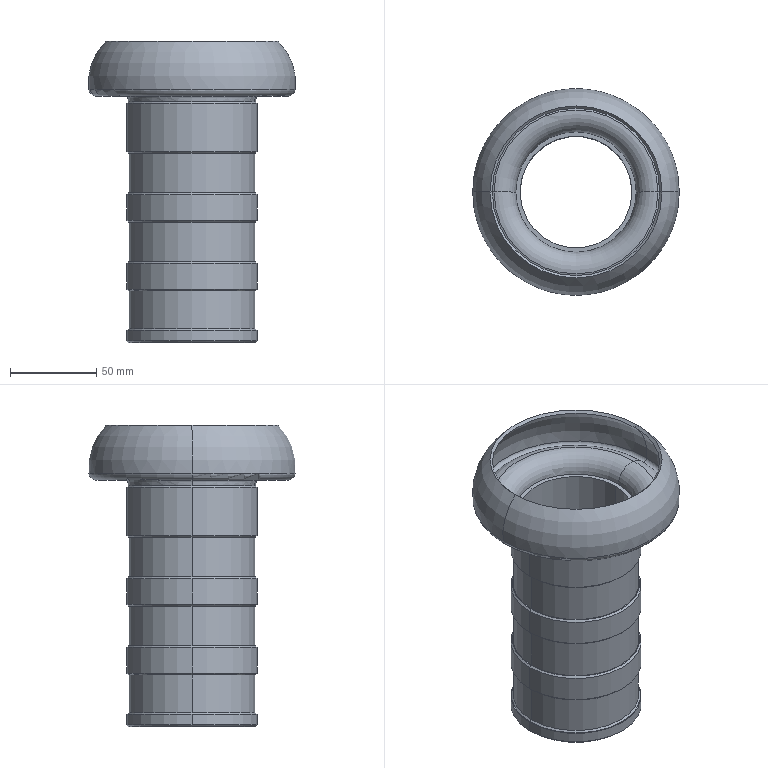Part | SolidWorks | features Chamfer 2, Extrusion 1, ICE 1, LPattern 1, Revolution 1 | 1 solid | 58 faces | box 120.458 x 120.458 x 175 mm | volume 185173 mm3 | cone 18 | torus 16 | cylinder 16 | plane 8 | commonest cylinder face diameters 76 x8 73 x6 65 x2
STEP:
#1=CARTESIAN_POINT('',(47.213,0.,148.274));
#2=VERTEX_POINT('',#1);
#3=CARTESIAN_POINT('',(-47.213,0.,148.274));
#4=VERTEX_POINT('',#3);
#5=CARTESIAN_POINT('',(0.,0.,148.274));
#6=DIRECTION('',(0.,0.,-1.));
#7=DIRECTION('',(-1.,0.,0.));
#8=AXIS2_PLACEMENT_3D('',#5,#6,#7);
#9=CIRCLE('',#8,47.213);
#10=EDGE_CURVE('',#2,#4,#9,.T.);
#11=ORIENTED_EDGE('',*,*,#10,.F.);
#12=CARTESIAN_POINT('',(54.205,0.,143.544));
#13=VERTEX_POINT('',#12);
#14=CARTESIAN_POINT('',(44.886,0.,137.301));
#15=DIRECTION('',(0.,1.,0.));
#16=DIRECTION('',(-1.,0.,0.));
#17=AXIS2_PLACEMENT_3D('',#14,#15,#16);
#18=CIRCLE('',#17,11.217);
#19=EDGE_CURVE('',#2,#13,#18,.T.);
#20=ORIENTED_EDGE('',*,*,#19,.T.);
#21=CARTESIAN_POINT('',(-54.205,0.,143.544));
#22=VERTEX_POINT('',#21);
#23=CARTESIAN_POINT('',(0.,0.,143.544));
#24=DIRECTION('',(0.,0.,-1.));
#25=DIRECTION('',(-1.,0.,0.));
#26=AXIS2_PLACEMENT_3D('',#23,#24,#25);
#27=CIRCLE('',#26,54.205);
#28=EDGE_CURVE('',#13,#22,#27,.T.);
#29=ORIENTED_EDGE('',*,*,#28,.T.);
#30=CARTESIAN_POINT('',(-44.886,0.,137.301));
#31=DIRECTION('',(0.,-1.,0.));
#32=DIRECTION('',(0.,0.,-1.));
#33=AXIS2_PLACEMENT_3D('',#30,#31,#32);
#34=CIRCLE('',#33,11.217);
#35=EDGE_CURVE('',#4,#22,#34,.T.);
#36=ORIENTED_EDGE('',*,*,#35,.F.);
#37=EDGE_LOOP('',(#11,#20,#29,#36));
#38=FACE_OUTER_BOUND('',#37,.T.);
#39=CARTESIAN_POINT('',(0.,0.,137.301));
#40=DIRECTION('',(0.,0.,-1.));
#41=DIRECTION('',(-1.,0.,0.));
#42=AXIS2_PLACEMENT_3D('',#39,#40,#41);
#43=TOROIDAL_SURFACE('',#42,44.886,11.217);
#44=ADVANCED_FACE('',(#38),#43,.F.);
#45=CARTESIAN_POINT('',(-60.,0.,147.099));
#46=VERTEX_POINT('',#45);
#47=CARTESIAN_POINT('',(60.,0.,147.099));
#48=VERTEX_POINT('',#47);
#49=CARTESIAN_POINT('',(0.,0.,147.099));
#50=DIRECTION('',(0.,0.,-1.));
#51=DIRECTION('',(-1.,0.,0.));
#52=AXIS2_PLACEMENT_3D('',#49,#50,#51);
#53=CIRCLE('',#52,60.);
#54=EDGE_CURVE('',#46,#48,#53,.T.);
#55=ORIENTED_EDGE('',*,*,#54,.T.);
#56=CARTESIAN_POINT('',(55.701,0.,147.606));
#57=DIRECTION('',(0.,1.,0.));
#58=DIRECTION('',(-1.,0.,0.));
#59=AXIS2_PLACEMENT_3D('',#56,#57,#58);
#60=CIRCLE('',#59,4.329);
#61=EDGE_CURVE('',#48,#13,#60,.T.);
#62=ORIENTED_EDGE('',*,*,#61,.T.);
#63=CARTESIAN_POINT('',(0.,0.,143.544));
#64=DIRECTION('',(0.,0.,-1.));
#65=DIRECTION('',(-1.,0.,0.));
#66=AXIS2_PLACEMENT_3D('',#63,#64,#65);
#67=CIRCLE('',#66,54.205);
#68=EDGE_CURVE('',#22,#13,#67,.T.);
#69=ORIENTED_EDGE('',*,*,#68,.F.);
#70=CARTESIAN_POINT('',(-55.701,0.,147.606));
#71=DIRECTION('',(0.,-1.,0.));
#72=DIRECTION('',(0.,0.,-1.));
#73=AXIS2_PLACEMENT_3D('',#70,#71,#72);
#74=CIRCLE('',#73,4.329);
#75=EDGE_CURVE('',#46,#22,#74,.T.);
#76=ORIENTED_EDGE('',*,*,#75,.F.);
#77=EDGE_LOOP('',(#55,#62,#69,#76));
#78=FACE_OUTER_BOUND('',#77,.T.);
#79=CARTESIAN_POINT('',(0.,0.,147.606));
#80=DIRECTION('',(0.,0.,-1.));
#81=DIRECTION('',(-1.,0.,0.));
#82=AXIS2_PLACEMENT_3D('',#79,#80,#81);
#83=TOROIDAL_SURFACE('',#82,55.701,4.329);
#84=ADVANCED_FACE('',(#78),#83,.T.);
#85=CARTESIAN_POINT('',(-50.,0.,175.));
#86=VERTEX_POINT('',#85);
#87=CARTESIAN_POINT('',(50.,0.,175.));
#88=VERTEX_POINT('',#87);
#89=CARTESIAN_POINT('',(0.,0.,175.));
#90=DIRECTION('',(0.,0.,-1.));
#91=DIRECTION('',(-1.,0.,0.));
#92=AXIS2_PLACEMENT_3D('',#89,#90,#91);
#93=CIRCLE('',#92,50.);
#94=EDGE_CURVE('',#86,#88,#93,.T.);
#95=ORIENTED_EDGE('',*,*,#94,.T.);
#96=CARTESIAN_POINT('',(26.951,0.,150.997));
#97=DIRECTION('',(0.,1.,0.));
#98=DIRECTION('',(-1.,0.,0.));
#99=AXIS2_PLACEMENT_3D('',#96,#97,#98);
#100=CIRCLE('',#99,33.278);
#101=EDGE_CURVE('',#88,#48,#100,.T.);
#102=ORIENTED_EDGE('',*,*,#101,.T.);
#103=ORIENTED_EDGE('',*,*,#54,.F.);
#104=CARTESIAN_POINT('',(-26.951,0.,150.997));
#105=DIRECTION('',(0.,-1.,0.));
#106=DIRECTION('',(0.,0.,-1.));
#107=AXIS2_PLACEMENT_3D('',#104,#105,#106);
#108=CIRCLE('',#107,33.278);
#109=EDGE_CURVE('',#86,#46,#108,.T.);
#110=ORIENTED_EDGE('',*,*,#109,.F.);
#111=EDGE_LOOP('',(#95,#102,#103,#110));
#112=FACE_OUTER_BOUND('',#111,.T.);
#113=CARTESIAN_POINT('',(0.,0.,150.997));
#114=DIRECTION('',(0.,0.,-1.));
#115=DIRECTION('',(-1.,0.,0.));
#116=AXIS2_PLACEMENT_3D('',#113,#114,#115);
#117=TOROIDAL_SURFACE('',#116,26.951,33.278);
#118=ADVANCED_FACE('',(#112),#117,.T.);
#119=CARTESIAN_POINT('',(48.615,0.,173.557));
#120=VERTEX_POINT('',#119);
#121=CARTESIAN_POINT('',(-48.615,0.,173.557));
#122=VERTEX_POINT('',#121);
#123=CARTESIAN_POINT('',(0.,0.,173.557));
#124=DIRECTION('',(0.,0.,-1.));
#125=DIRECTION('',(-1.,0.,0.));
#126=AXIS2_PLACEMENT_3D('',#123,#124,#125);
#127=CIRCLE('',#126,48.615);
#128=EDGE_CURVE('',#120,#122,#127,.T.);
#129=ORIENTED_EDGE('',*,*,#128,.T.);
#130=CARTESIAN_POINT('',(-48.615,0.,173.557));
#131=DIRECTION('',(-0.6926,0.,0.7213));
#132=VECTOR('',#131,1000.);
#133=LINE('',#130,#132);
#134=EDGE_CURVE('',#122,#86,#133,.T.);
#135=ORIENTED_EDGE('',*,*,#134,.T.);
#136=CARTESIAN_POINT('',(0.,0.,175.));
#137=DIRECTION('',(0.,0.,-1.));
#138=DIRECTION('',(-1.,0.,0.));
#139=AXIS2_PLACEMENT_3D('',#136,#137,#138);
#140=CIRCLE('',#139,50.);
#141=EDGE_CURVE('',#88,#86,#140,.T.);
#142=ORIENTED_EDGE('',*,*,#141,.F.);
#143=CARTESIAN_POINT('',(48.615,0.,173.557));
#144=DIRECTION('',(0.6926,0.,0.7213));
#145=VECTOR('',#144,1000.);
#146=LINE('',#143,#145);
#147=EDGE_CURVE('',#120,#88,#146,.T.);
#148=ORIENTED_EDGE('',*,*,#147,.F.);
#149=EDGE_LOOP('',(#129,#135,#142,#148));
#150=FACE_OUTER_BOUND('',#149,.T.);
#151=CARTESIAN_POINT('',(0.,0.,173.557));
#152=DIRECTION('',(0.,0.,1.));
#153=DIRECTION('',(1.,0.,0.));
#154=AXIS2_PLACEMENT_3D('',#151,#152,#153);
#155=CONICAL_SURFACE('',#154,48.615,0.7651);
#156=ADVANCED_FACE('',(#150),#155,.F.);
#157=ORIENTED_EDGE('',*,*,#128,.F.);
#158=CARTESIAN_POINT('',(58.014,0.,147.333));
#159=VERTEX_POINT('',#158);
#160=CARTESIAN_POINT('',(26.951,0.,150.997));
#161=DIRECTION('',(0.,1.,0.));
#162=DIRECTION('',(-1.,0.,0.));
#163=AXIS2_PLACEMENT_3D('',#160,#161,#162);
#164=CIRCLE('',#163,31.278);
#165=EDGE_CURVE('',#120,#159,#164,.T.);
#166=ORIENTED_EDGE('',*,*,#165,.T.);
#167=CARTESIAN_POINT('',(-58.014,0.,147.333));
#168=VERTEX_POINT('',#167);
#169=CARTESIAN_POINT('',(0.,0.,147.333));
#170=DIRECTION('',(0.,0.,-1.));
#171=DIRECTION('',(-1.,0.,0.));
#172=AXIS2_PLACEMENT_3D('',#169,#170,#171);
#173=CIRCLE('',#172,58.014);
#174=EDGE_CURVE('',#159,#168,#173,.T.);
#175=ORIENTED_EDGE('',*,*,#174,.T.);
#176=CARTESIAN_POINT('',(-26.951,0.,150.997));
#177=DIRECTION('',(0.,-1.,0.));
#178=DIRECTION('',(0.,0.,-1.));
#179=AXIS2_PLACEMENT_3D('',#176,#177,#178);
#180=CIRCLE('',#179,31.278);
#181=EDGE_CURVE('',#122,#168,#180,.T.);
#182=ORIENTED_EDGE('',*,*,#181,.F.);
#183=EDGE_LOOP('',(#157,#166,#175,#182));
#184=FACE_OUTER_BOUND('',#183,.T.);
#185=CARTESIAN_POINT('',(0.,0.,150.997));
#186=DIRECTION('',(0.,0.,-1.));
#187=DIRECTION('',(-1.,0.,0.));
#188=AXIS2_PLACEMENT_3D('',#185,#186,#187);
#189=TOROIDAL_SURFACE('',#188,26.951,31.278);
#190=ADVANCED_FACE('',(#184),#189,.F.);
#191=ORIENTED_EDGE('',*,*,#174,.F.);
#192=CARTESIAN_POINT('',(55.411,0.,145.295));
#193=VERTEX_POINT('',#192);
#194=CARTESIAN_POINT('',(55.701,0.,147.606));
#195=DIRECTION('',(0.,1.,0.));
#196=DIRECTION('',(-1.,0.,0.));
#197=AXIS2_PLACEMENT_3D('',#194,#195,#196);
#198=CIRCLE('',#197,2.329);
#199=EDGE_CURVE('',#159,#193,#198,.T.);
#200=ORIENTED_EDGE('',*,*,#199,.T.);
#201=CARTESIAN_POINT('',(-55.411,0.,145.295));
#202=VERTEX_POINT('',#201);
#203=CARTESIAN_POINT('',(0.,0.,145.295));
#204=DIRECTION('',(0.,0.,-1.));
#205=DIRECTION('',(-1.,0.,0.));
#206=AXIS2_PLACEMENT_3D('',#203,#204,#205);
#207=CIRCLE('',#206,55.411);
#208=EDGE_CURVE('',#193,#202,#207,.T.);
#209=ORIENTED_EDGE('',*,*,#208,.T.);
#210=CARTESIAN_POINT('',(-55.701,0.,147.606));
#211=DIRECTION('',(0.,-1.,0.));
#212=DIRECTION('',(0.,0.,-1.));
#213=AXIS2_PLACEMENT_3D('',#210,#211,#212);
#214=CIRCLE('',#213,2.329);
#215=EDGE_CURVE('',#168,#202,#214,.T.);
#216=ORIENTED_EDGE('',*,*,#215,.F.);
#217=EDGE_LOOP('',(#191,#200,#209,#216));
#218=FACE_OUTER_BOUND('',#217,.T.);
#219=CARTESIAN_POINT('',(0.,0.,147.606));
#220=DIRECTION('',(0.,0.,-1.));
#221=DIRECTION('',(-1.,0.,0.));
#222=AXIS2_PLACEMENT_3D('',#219,#220,#221);
#223=TOROIDAL_SURFACE('',#222,55.701,2.329);
#224=ADVANCED_FACE('',(#218),#223,.F.);
#225=CARTESIAN_POINT('',(-47.628,0.,150.231));
#226=VERTEX_POINT('',#225);
#227=CARTESIAN_POINT('',(47.628,0.,150.231));
#228=VERTEX_POINT('',#227);
#229=CARTESIAN_POINT('',(0.,0.,150.231));
#230=DIRECTION('',(0.,0.,-1.));
#231=DIRECTION('',(-1.,0.,0.));
#232=AXIS2_PLACEMENT_3D('',#229,#230,#231);
#233=CIRCLE('',#232,47.628);
#234=EDGE_CURVE('',#226,#228,#233,.T.);
#235=ORIENTED_EDGE('',*,*,#234,.T.);
#236=CARTESIAN_POINT('',(44.886,0.,137.301));
#237=DIRECTION('',(0.,1.,0.));
#238=DIRECTION('',(-1.,0.,0.));
#239=AXIS2_PLACEMENT_3D('',#236,#237,#238);
#240=CIRCLE('',#239,13.217);
#241=EDGE_CURVE('',#228,#193,#240,.T.);
#242=ORIENTED_EDGE('',*,*,#241,.T.);
#243=CARTESIAN_POINT('',(0.,0.,145.295));
#244=DIRECTION('',(0.,0.,-1.));
#245=DIRECTION('',(-1.,0.,0.));
#246=AXIS2_PLACEMENT_3D('',#243,#244,#245);
#247=CIRCLE('',#246,55.411);
#248=EDGE_CURVE('',#202,#193,#247,.T.);
#249=ORIENTED_EDGE('',*,*,#248,.F.);
#250=CARTESIAN_POINT('',(-44.886,0.,137.301));
#251=DIRECTION('',(0.,-1.,0.));
#252=DIRECTION('',(0.,0.,-1.));
#253=AXIS2_PLACEMENT_3D('',#250,#251,#252);
#254=CIRCLE('',#253,13.217);
#255=EDGE_CURVE('',#226,#202,#254,.T.);
#256=ORIENTED_EDGE('',*,*,#255,.F.);
#257=EDGE_LOOP('',(#235,#242,#249,#256));
#258=FACE_OUTER_BOUND('',#257,.T.);
#259=CARTESIAN_POINT('',(0.,0.,137.301));
#260=DIRECTION('',(0.,0.,-1.));
#261=DIRECTION('',(-1.,0.,0.));
#262=AXIS2_PLACEMENT_3D('',#259,#260,#261);
#263=TOROIDAL_SURFACE('',#262,44.886,13.217);
#264=ADVANCED_FACE('',(#258),#263,.T.);
#265=CARTESIAN_POINT('',(-35.,0.,140.));
#266=VERTEX_POINT('',#265);
#267=CARTESIAN_POINT('',(35.,0.,140.));
#268=VERTEX_POINT('',#267);
#269=CARTESIAN_POINT('',(0.,0.,140.));
#270=DIRECTION('',(0.,0.,-1.));
#271=DIRECTION('',(-1.,0.,0.));
#272=AXIS2_PLACEMENT_3D('',#269,#270,#271);
#273=CIRCLE('',#272,35.);
#274=EDGE_CURVE('',#266,#268,#273,.T.);
#275=ORIENTED_EDGE('',*,*,#274,.T.);
#276=CARTESIAN_POINT('',(45.458,0.,140.));
#277=DIRECTION('',(0.,1.,0.));
#278=DIRECTION('',(-1.,0.,0.));
#279=AXIS2_PLACEMENT_3D('',#276,#277,#278);
#280=CIRCLE('',#279,10.458);
#281=EDGE_CURVE('',#268,#228,#280,.T.);
#282=ORIENTED_EDGE('',*,*,#281,.T.);
#283=ORIENTED_EDGE('',*,*,#234,.F.);
#284=CARTESIAN_POINT('',(-45.458,0.,140.));
#285=DIRECTION('',(0.,-1.,0.));
#286=DIRECTION('',(0.,0.,-1.));
#287=AXIS2_PLACEMENT_3D('',#284,#285,#286);
#288=CIRCLE('',#287,10.458);
#289=EDGE_CURVE('',#266,#226,#288,.T.);
#290=ORIENTED_EDGE('',*,*,#289,.F.);
#291=EDGE_LOOP('',(#275,#282,#283,#290));
#292=FACE_OUTER_BOUND('',#291,.T.);
#293=CARTESIAN_POINT('',(0.,0.,140.));
#294=DIRECTION('',(0.,0.,-1.));
#295=DIRECTION('',(-1.,0.,0.));
#296=AXIS2_PLACEMENT_3D('',#293,#294,#295);
#297=TOROIDAL_SURFACE('',#296,45.458,10.458);
#298=ADVANCED_FACE('',(#292),#297,.T.);
#299=CARTESIAN_POINT('',(-37.,0.,140.));
#300=VERTEX_POINT('',#299);
#301=CARTESIAN_POINT('',(37.,0.,140.));
#302=VERTEX_POINT('',#301);
#303=CARTESIAN_POINT('',(0.,0.,140.));
#304=DIRECTION('',(0.,0.,1.));
#305=DIRECTION('',(1.,0.,0.));
#306=AXIS2_PLACEMENT_3D('',#303,#304,#305);
#307=CIRCLE('',#306,37.);
#308=EDGE_CURVE('',#300,#302,#307,.T.);
#309=ORIENTED_EDGE('',*,*,#308,.T.);
#310=CARTESIAN_POINT('',(45.458,0.,140.));
#311=DIRECTION('',(0.,1.,0.));
#312=DIRECTION('',(-1.,0.,0.));
#313=AXIS2_PLACEMENT_3D('',#310,#311,#312);
#314=CIRCLE('',#313,8.458);
#315=EDGE_CURVE('',#302,#2,#314,.T.);
#316=ORIENTED_EDGE('',*,*,#315,.T.);
#317=ORIENTED_EDGE('',*,*,#10,.T.);
#318=CARTESIAN_POINT('',(-45.458,0.,140.));
#319=DIRECTION('',(0.,-1.,0.));
#320=DIRECTION('',(0.,0.,-1.));
#321=AXIS2_PLACEMENT_3D('',#318,#319,#320);
#322=CIRCLE('',#321,8.458);
#323=EDGE_CURVE('',#300,#4,#322,.T.);
#324=ORIENTED_EDGE('',*,*,#323,.F.);
#325=EDGE_LOOP('',(#309,#316,#317,#324));
#326=FACE_OUTER_BOUND('',#325,.T.);
#327=CARTESIAN_POINT('',(0.,0.,140.));
#328=DIRECTION('',(0.,0.,-1.));
#329=DIRECTION('',(-1.,0.,0.));
#330=AXIS2_PLACEMENT_3D('',#327,#328,#329);
#331=TOROIDAL_SURFACE('',#330,45.458,8.458);
#332=ADVANCED_FACE('',(#326),#331,.F.);
#333=CARTESIAN_POINT('',(-37.,0.,110.));
#334=VERTEX_POINT('',#333);
#335=CARTESIAN_POINT('',(37.,0.,110.));
#336=VERTEX_POINT('',#335);
#337=CARTESIAN_POINT('',(0.,0.,110.));
#338=DIRECTION('',(0.,0.,-1.));
#339=DIRECTION('',(1.,0.,0.));
#340=AXIS2_PLACEMENT_3D('',#337,#338,#339);
#341=CIRCLE('',#340,37.);
#342=EDGE_CURVE('',#334,#336,#341,.T.);
#343=ORIENTED_EDGE('',*,*,#342,.F.);
#344=CARTESIAN_POINT('',(-38.,0.,111.));
#345=VERTEX_POINT('',#344);
#346=CARTESIAN_POINT('',(-38.,0.,111.));
#347=DIRECTION('',(-0.7071,0.,0.7071));
#348=VECTOR('',#347,1000.);
#349=LINE('',#346,#348);
#350=EDGE_CURVE('',#334,#345,#349,.T.);
#351=ORIENTED_EDGE('',*,*,#350,.T.);
#352=CARTESIAN_POINT('',(38.,0.,111.));
#353=VERTEX_POINT('',#352);
#354=CARTESIAN_POINT('',(0.,0.,111.));
#355=DIRECTION('',(0.,0.,1.));
#356=DIRECTION('',(1.,0.,0.));
#357=AXIS2_PLACEMENT_3D('',#354,#355,#356);
#358=CIRCLE('',#357,38.);
#359=EDGE_CURVE('',#353,#345,#358,.T.);
#360=ORIENTED_EDGE('',*,*,#359,.F.);
#361=CARTESIAN_POINT('',(38.,0.,111.));
#362=DIRECTION('',(0.7071,0.,0.7071));
#363=VECTOR('',#362,1000.);
#364=LINE('',#361,#363);
#365=EDGE_CURVE('',#336,#353,#364,.T.);
#366=ORIENTED_EDGE('',*,*,#365,.F.);
#367=EDGE_LOOP('',(#343,#351,#360,#366));
#368=FACE_OUTER_BOUND('',#367,.T.);
#369=CARTESIAN_POINT('',(0.,0.,111.));
#370=DIRECTION('',(0.,0.,1.));
#371=DIRECTION('',(1.,0.,0.));
#372=AXIS2_PLACEMENT_3D('',#369,#370,#371);
#373=CONICAL_SURFACE('',#372,38.,0.7854);
#374=ADVANCED_FACE('',(#368),#373,.T.);
#375=CARTESIAN_POINT('',(37.,0.,87.));
#376=VERTEX_POINT('',#375);
#377=CARTESIAN_POINT('',(-37.,0.,87.));
#378=VERTEX_POINT('',#377);
#379=CARTESIAN_POINT('',(0.,0.,87.));
#380=DIRECTION('',(0.,0.,1.));
#381=DIRECTION('',(1.,0.,0.));
#382=AXIS2_PLACEMENT_3D('',#379,#380,#381);
#383=CIRCLE('',#382,37.);
#384=EDGE_CURVE('',#376,#378,#383,.T.);
#385=ORIENTED_EDGE('',*,*,#384,.F.);
#386=CARTESIAN_POINT('',(38.,0.,86.));
#387=VERTEX_POINT('',#386);
#388=CARTESIAN_POINT('',(37.,0.,87.));
#389=DIRECTION('',(0.7071,0.,-0.7071));
#390=VECTOR('',#389,1000.);
#391=LINE('',#388,#390);
#392=EDGE_CURVE('',#376,#387,#391,.T.);
#393=ORIENTED_EDGE('',*,*,#392,.T.);
#394=CARTESIAN_POINT('',(-38.,0.,86.));
#395=VERTEX_POINT('',#394);
#396=CARTESIAN_POINT('',(0.,0.,86.));
#397=DIRECTION('',(0.,0.,-1.));
#398=DIRECTION('',(1.,0.,0.));
#399=AXIS2_PLACEMENT_3D('',#396,#397,#398);
#400=CIRCLE('',#399,38.);
#401=EDGE_CURVE('',#395,#387,#400,.T.);
#402=ORIENTED_EDGE('',*,*,#401,.F.);
#403=CARTESIAN_POINT('',(-37.,0.,87.));
#404=DIRECTION('',(-0.7071,0.,-0.7071));
#405=VECTOR('',#404,1000.);
#406=LINE('',#403,#405);
#407=EDGE_CURVE('',#378,#395,#406,.T.);
#408=ORIENTED_EDGE('',*,*,#407,.F.);
#409=EDGE_LOOP('',(#385,#393,#402,#408));
#410=FACE_OUTER_BOUND('',#409,.T.);
#411=CARTESIAN_POINT('',(0.,0.,87.));
#412=DIRECTION('',(0.,0.,-1.));
#413=DIRECTION('',(-1.,0.,0.));
#414=AXIS2_PLACEMENT_3D('',#411,#412,#413);
#415=CONICAL_SURFACE('',#414,37.,0.7854);
#416=ADVANCED_FACE('',(#410),#415,.T.);
#417=CARTESIAN_POINT('',(-37.,0.,70.));
#418=VERTEX_POINT('',#417);
#419=CARTESIAN_POINT('',(37.,0.,70.));
#420=VERTEX_POINT('',#419);
#421=CARTESIAN_POINT('',(0.,0.,70.));
#422=DIRECTION('',(0.,0.,-1.));
#423=DIRECTION('',(1.,0.,0.));
#424=AXIS2_PLACEMENT_3D('',#421,#422,#423);
#425=CIRCLE('',#424,37.);
#426=EDGE_CURVE('',#418,#420,#425,.T.);
#427=ORIENTED_EDGE('',*,*,#426,.F.);
#428=CARTESIAN_POINT('',(-38.,0.,71.));
#429=VERTEX_POINT('',#428);
#430=CARTESIAN_POINT('',(-38.,0.,71.));
#431=DIRECTION('',(-0.7071,0.,0.7071));
#432=VECTOR('',#431,1000.);
#433=LINE('',#430,#432);
#434=EDGE_CURVE('',#418,#429,#433,.T.);
#435=ORIENTED_EDGE('',*,*,#434,.T.);
#436=CARTESIAN_POINT('',(38.,0.,71.));
#437=VERTEX_POINT('',#436);
#438=CARTESIAN_POINT('',(0.,0.,71.));
#439=DIRECTION('',(0.,0.,1.));
#440=DIRECTION('',(1.,0.,0.));
#441=AXIS2_PLACEMENT_3D('',#438,#439,#440);
#442=CIRCLE('',#441,38.);
#443=EDGE_CURVE('',#437,#429,#442,.T.);
#444=ORIENTED_EDGE('',*,*,#443,.F.);
#445=CARTESIAN_POINT('',(38.,0.,71.));
#446=DIRECTION('',(0.7071,0.,0.7071));
#447=VECTOR('',#446,1000.);
#448=LINE('',#445,#447);
#449=EDGE_CURVE('',#420,#437,#448,.T.);
#450=ORIENTED_EDGE('',*,*,#449,.F.);
#451=EDGE_LOOP('',(#427,#435,#444,#450));
#452=FACE_OUTER_BOUND('',#451,.T.);
#453=CARTESIAN_POINT('',(0.,0.,71.));
#454=DIRECTION('',(0.,0.,1.));
#455=DIRECTION('',(1.,0.,0.));
#456=AXIS2_PLACEMENT_3D('',#453,#454,#455);
#457=CONICAL_SURFACE('',#456,38.,0.7854);
#458=ADVANCED_FACE('',(#452),#457,.T.);
#459=CARTESIAN_POINT('',(37.,0.,47.));
#460=VERTEX_POINT('',#459);
#461=CARTESIAN_POINT('',(-37.,0.,47.));
#462=VERTEX_POINT('',#461);
#463=CARTESIAN_POINT('',(0.,0.,47.));
#464=DIRECTION('',(0.,0.,1.));
#465=DIRECTION('',(1.,0.,0.));
#466=AXIS2_PLACEMENT_3D('',#463,#464,#465);
#467=CIRCLE('',#466,37.);
#468=EDGE_CURVE('',#460,#462,#467,.T.);
#469=ORIENTED_EDGE('',*,*,#468,.F.);
#470=CARTESIAN_POINT('',(38.,0.,46.));
#471=VERTEX_POINT('',#470);
#472=CARTESIAN_POINT('',(37.,0.,47.));
#473=DIRECTION('',(0.7071,0.,-0.7071));
#474=VECTOR('',#473,1000.);
#475=LINE('',#472,#474);
#476=EDGE_CURVE('',#460,#471,#475,.T.);
#477=ORIENTED_EDGE('',*,*,#476,.T.);
#478=CARTESIAN_POINT('',(-38.,0.,46.));
#479=VERTEX_POINT('',#478);
#480=CARTESIAN_POINT('',(0.,0.,46.));
#481=DIRECTION('',(0.,0.,-1.));
#482=DIRECTION('',(1.,0.,0.));
#483=AXIS2_PLACEMENT_3D('',#480,#481,#482);
#484=CIRCLE('',#483,38.);
#485=EDGE_CURVE('',#479,#471,#484,.T.);
#486=ORIENTED_EDGE('',*,*,#485,.F.);
#487=CARTESIAN_POINT('',(-37.,0.,47.));
#488=DIRECTION('',(-0.7071,0.,-0.7071));
#489=VECTOR('',#488,1000.);
#490=LINE('',#487,#489);
#491=EDGE_CURVE('',#462,#479,#490,.T.);
#492=ORIENTED_EDGE('',*,*,#491,.F.);
#493=EDGE_LOOP('',(#469,#477,#486,#492));
#494=FACE_OUTER_BOUND('',#493,.T.);
#495=CARTESIAN_POINT('',(0.,0.,47.));
#496=DIRECTION('',(0.,0.,-1.));
#497=DIRECTION('',(-1.,0.,0.));
#498=AXIS2_PLACEMENT_3D('',#495,#496,#497);
#499=CONICAL_SURFACE('',#498,37.,0.7854);
#500=ADVANCED_FACE('',(#494),#499,.T.);
#501=CARTESIAN_POINT('',(-37.,0.,30.));
#502=VERTEX_POINT('',#501);
#503=CARTESIAN_POINT('',(37.,0.,30.));
#504=VERTEX_POINT('',#503);
#505=CARTESIAN_POINT('',(0.,0.,30.));
#506=DIRECTION('',(0.,0.,-1.));
#507=DIRECTION('',(1.,0.,0.));
#508=AXIS2_PLACEMENT_3D('',#505,#506,#507);
#509=CIRCLE('',#508,37.);
#510=EDGE_CURVE('',#502,#504,#509,.T.);
#511=ORIENTED_EDGE('',*,*,#510,.F.);
#512=CARTESIAN_POINT('',(-38.,0.,31.));
#513=VERTEX_POINT('',#512);
#514=CARTESIAN_POINT('',(-38.,0.,31.));
#515=DIRECTION('',(-0.7071,0.,0.7071));
#516=VECTOR('',#515,1000.);
#517=LINE('',#514,#516);
#518=EDGE_CURVE('',#502,#513,#517,.T.);
#519=ORIENTED_EDGE('',*,*,#518,.T.);
#520=CARTESIAN_POINT('',(38.,0.,31.));
#521=VERTEX_POINT('',#520);
#522=CARTESIAN_POINT('',(0.,0.,31.));
#523=DIRECTION('',(0.,0.,1.));
#524=DIRECTION('',(1.,0.,0.));
#525=AXIS2_PLACEMENT_3D('',#522,#523,#524);
#526=CIRCLE('',#525,38.);
#527=EDGE_CURVE('',#521,#513,#526,.T.);
#528=ORIENTED_EDGE('',*,*,#527,.F.);
#529=CARTESIAN_POINT('',(38.,0.,31.));
#530=DIRECTION('',(0.7071,0.,0.7071));
#531=VECTOR('',#530,1000.);
#532=LINE('',#529,#531);
#533=EDGE_CURVE('',#504,#521,#532,.T.);
#534=ORIENTED_EDGE('',*,*,#533,.F.);
#535=EDGE_LOOP('',(#511,#519,#528,#534));
#536=FACE_OUTER_BOUND('',#535,.T.);
#537=CARTESIAN_POINT('',(0.,0.,31.));
#538=DIRECTION('',(0.,0.,1.));
#539=DIRECTION('',(1.,0.,0.));
#540=AXIS2_PLACEMENT_3D('',#537,#538,#539);
#541=CONICAL_SURFACE('',#540,38.,0.7854);
#542=ADVANCED_FACE('',(#536),#541,.T.);
#543=CARTESIAN_POINT('',(36.5,0.,8.));
#544=VERTEX_POINT('',#543);
#545=CARTESIAN_POINT('',(-36.5,0.,8.));
#546=VERTEX_POINT('',#545);
#547=CARTESIAN_POINT('',(0.,0.,8.));
#548=DIRECTION('',(0.,0.,1.));
#549=DIRECTION('',(1.,0.,0.));
#550=AXIS2_PLACEMENT_3D('',#547,#548,#549);
#551=CIRCLE('',#550,36.5);
#552=EDGE_CURVE('',#544,#546,#551,.T.);
#553=ORIENTED_EDGE('',*,*,#552,.F.);
#554=CARTESIAN_POINT('',(37.5,0.,7.));
#555=VERTEX_POINT('',#554);
#556=CARTESIAN_POINT('',(36.5,0.,8.));
#557=DIRECTION('',(0.7071,0.,-0.7071));
#558=VECTOR('',#557,1000.);
#559=LINE('',#556,#558);
#560=EDGE_CURVE('',#544,#555,#559,.T.);
#561=ORIENTED_EDGE('',*,*,#560,.T.);
#562=CARTESIAN_POINT('',(-37.5,0.,7.));
#563=VERTEX_POINT('',#562);
#564=CARTESIAN_POINT('',(0.,0.,7.));
#565=DIRECTION('',(0.,0.,-1.));
#566=DIRECTION('',(1.,0.,0.));
#567=AXIS2_PLACEMENT_3D('',#564,#565,#566);
#568=CIRCLE('',#567,37.5);
#569=EDGE_CURVE('',#563,#555,#568,.T.);
#570=ORIENTED_EDGE('',*,*,#569,.F.);
#571=CARTESIAN_POINT('',(-36.5,0.,8.));
#572=DIRECTION('',(-0.7071,0.,-0.7071));
#573=VECTOR('',#572,1000.);
#574=LINE('',#571,#573);
#575=EDGE_CURVE('',#546,#563,#574,.T.);
#576=ORIENTED_EDGE('',*,*,#575,.F.);
#577=EDGE_LOOP('',(#553,#561,#570,#576));
#578=FACE_OUTER_BOUND('',#577,.T.);
#579=CARTESIAN_POINT('',(0.,0.,8.));
#580=DIRECTION('',(0.,0.,-1.));
#581=DIRECTION('',(-1.,0.,0.));
#582=AXIS2_PLACEMENT_3D('',#579,#580,#581);
#583=CONICAL_SURFACE('',#582,36.5,0.7854);
#584=ADVANCED_FACE('',(#578),#583,.T.);
#585=CARTESIAN_POINT('',(-37.,0.,0.));
#586=VERTEX_POINT('',#585);
#587=CARTESIAN_POINT('',(37.,0.,0.));
#588=VERTEX_POINT('',#587);
#589=CARTESIAN_POINT('',(0.,0.,0.));
#590=DIRECTION('',(0.,0.,-1.));
#591=DIRECTION('',(1.,0.,0.));
#592=AXIS2_PLACEMENT_3D('',#589,#590,#591);
#593=CIRCLE('',#592,37.);
#594=EDGE_CURVE('',#586,#588,#593,.T.);
#595=ORIENTED_EDGE('',*,*,#594,.F.);
#596=CARTESIAN_POINT('',(-38.,0.,1.));
#597=VERTEX_POINT('',#596);
#598=CARTESIAN_POINT('',(-38.,0.,1.));
#599=DIRECTION('',(-0.7071,0.,0.7071));
#600=VECTOR('',#599,1000.);
#601=LINE('',#598,#600);
#602=EDGE_CURVE('',#586,#597,#601,.T.);
#603=ORIENTED_EDGE('',*,*,#602,.T.);
#604=CARTESIAN_POINT('',(38.,0.,1.));
#605=VERTEX_POINT('',#604);
#606=CARTESIAN_POINT('',(0.,0.,1.));
#607=DIRECTION('',(0.,0.,1.));
#608=DIRECTION('',(1.,0.,0.));
#609=AXIS2_PLACEMENT_3D('',#606,#607,#608);
#610=CIRCLE('',#609,38.);
#611=EDGE_CURVE('',#605,#597,#610,.T.);
#612=ORIENTED_EDGE('',*,*,#611,.F.);
#613=CARTESIAN_POINT('',(38.,0.,1.));
#614=DIRECTION('',(0.7071,0.,0.7071));
#615=VECTOR('',#614,1000.);
#616=LINE('',#613,#615);
#617=EDGE_CURVE('',#588,#605,#616,.T.);
#618=ORIENTED_EDGE('',*,*,#617,.F.);
#619=EDGE_LOOP('',(#595,#603,#612,#618));
#620=FACE_OUTER_BOUND('',#619,.T.);
#621=CARTESIAN_POINT('',(0.,0.,1.));
#622=DIRECTION('',(0.,0.,1.));
#623=DIRECTION('',(1.,0.,0.));
#624=AXIS2_PLACEMENT_3D('',#621,#622,#623);
#625=CONICAL_SURFACE('',#624,38.,0.7854);
#626=ADVANCED_FACE('',(#620),#625,.T.);
#627=ORIENTED_EDGE('',*,*,#485,.T.);
#628=CARTESIAN_POINT('',(38.,0.,140.));
#629=DIRECTION('',(0.,0.,-1.));
#630=VECTOR('',#629,1000.);
#631=LINE('',#628,#630);
#632=EDGE_CURVE('',#471,#521,#631,.T.);
#633=ORIENTED_EDGE('',*,*,#632,.T.);
#634=ORIENTED_EDGE('',*,*,#527,.T.);
#635=CARTESIAN_POINT('',(-38.,0.,140.));
#636=DIRECTION('',(0.,0.,-1.));
#637=VECTOR('',#636,1000.);
#638=LINE('',#635,#637);
#639=EDGE_CURVE('',#479,#513,#638,.T.);
#640=ORIENTED_EDGE('',*,*,#639,.F.);
#641=EDGE_LOOP('',(#627,#633,#634,#640));
#642=FACE_OUTER_BOUND('',#641,.T.);
#643=CARTESIAN_POINT('',(0.,0.,140.));
#644=DIRECTION('',(0.,0.,-1.));
#645=DIRECTION('',(-1.,0.,0.));
#646=AXIS2_PLACEMENT_3D('',#643,#644,#645);
#647=CYLINDRICAL_SURFACE('',#646,38.);
#648=ADVANCED_FACE('',(#642),#647,.T.);
#649=CARTESIAN_POINT('',(36.5,0.,47.));
#650=VERTEX_POINT('',#649);
#651=CARTESIAN_POINT('',(-36.5,0.,47.));
#652=VERTEX_POINT('',#651);
#653=CARTESIAN_POINT('',(0.,0.,47.));
#654=DIRECTION('',(0.,0.,1.));
#655=DIRECTION('',(1.,0.,0.));
#656=AXIS2_PLACEMENT_3D('',#653,#654,#655);
#657=CIRCLE('',#656,36.5);
#658=EDGE_CURVE('',#650,#652,#657,.T.);
#659=ORIENTED_EDGE('',*,*,#658,.T.);
#660=CARTESIAN_POINT('',(-36.5,0.,70.));
#661=VERTEX_POINT('',#660);
#662=CARTESIAN_POINT('',(-36.5,0.,47.));
#663=DIRECTION('',(0.,0.,1.));
#664=VECTOR('',#663,1000.);
#665=LINE('',#662,#664);
#666=EDGE_CURVE('',#652,#661,#665,.T.);
#667=ORIENTED_EDGE('',*,*,#666,.T.);
#668=CARTESIAN_POINT('',(36.5,0.,70.));
#669=VERTEX_POINT('',#668);
#670=CARTESIAN_POINT('',(0.,0.,70.));
#671=DIRECTION('',(0.,0.,1.));
#672=DIRECTION('',(1.,0.,0.));
#673=AXIS2_PLACEMENT_3D('',#670,#671,#672);
#674=CIRCLE('',#673,36.5);
#675=EDGE_CURVE('',#669,#661,#674,.T.);
#676=ORIENTED_EDGE('',*,*,#675,.F.);
#677=CARTESIAN_POINT('',(36.5,0.,47.));
#678=DIRECTION('',(0.,0.,1.));
#679=VECTOR('',#678,1000.);
#680=LINE('',#677,#679);
#681=EDGE_CURVE('',#650,#669,#680,.T.);
#682=ORIENTED_EDGE('',*,*,#681,.F.);
#683=EDGE_LOOP('',(#659,#667,#676,#682));
#684=FACE_OUTER_BOUND('',#683,.T.);
#685=CARTESIAN_POINT('',(0.,0.,47.));
#686=DIRECTION('',(0.,0.,1.));
#687=DIRECTION('',(1.,0.,0.));
#688=AXIS2_PLACEMENT_3D('',#685,#686,#687);
#689=CYLINDRICAL_SURFACE('',#688,36.5);
#690=ADVANCED_FACE('',(#684),#689,.T.);
#691=ORIENTED_EDGE('',*,*,#552,.T.);
#692=CARTESIAN_POINT('',(-36.5,0.,30.));
#693=VERTEX_POINT('',#692);
#694=CARTESIAN_POINT('',(-36.5,0.,7.));
#695=DIRECTION('',(0.,0.,1.));
#696=VECTOR('',#695,1000.);
#697=LINE('',#694,#696);
#698=EDGE_CURVE('',#546,#693,#697,.T.);
#699=ORIENTED_EDGE('',*,*,#698,.T.);
#700=CARTESIAN_POINT('',(36.5,0.,30.));
#701=VERTEX_POINT('',#700);
#702=CARTESIAN_POINT('',(0.,0.,30.));
#703=DIRECTION('',(0.,0.,1.));
#704=DIRECTION('',(1.,0.,0.));
#705=AXIS2_PLACEMENT_3D('',#702,#703,#704);
#706=CIRCLE('',#705,36.5);
#707=EDGE_CURVE('',#701,#693,#706,.T.);
#708=ORIENTED_EDGE('',*,*,#707,.F.);
#709=CARTESIAN_POINT('',(36.5,0.,7.));
#710=DIRECTION('',(0.,0.,1.));
#711=VECTOR('',#710,1000.);
#712=LINE('',#709,#711);
#713=EDGE_CURVE('',#544,#701,#712,.T.);
#714=ORIENTED_EDGE('',*,*,#713,.F.);
#715=EDGE_LOOP('',(#691,#699,#708,#714));
#716=FACE_OUTER_BOUND('',#715,.T.);
#717=CARTESIAN_POINT('',(0.,0.,7.));
#718=DIRECTION('',(0.,0.,1.));
#719=DIRECTION('',(1.,0.,0.));
#720=AXIS2_PLACEMENT_3D('',#717,#718,#719);
#721=CYLINDRICAL_SURFACE('',#720,36.5);
#722=ADVANCED_FACE('',(#716),#721,.T.);
#723=CARTESIAN_POINT('',(36.5,0.,87.));
#724=VERTEX_POINT('',#723);
#725=CARTESIAN_POINT('',(-36.5,0.,87.));
#726=VERTEX_POINT('',#725);
#727=CARTESIAN_POINT('',(0.,0.,87.));
#728=DIRECTION('',(0.,0.,1.));
#729=DIRECTION('',(1.,0.,0.));
#730=AXIS2_PLACEMENT_3D('',#727,#728,#729);
#731=CIRCLE('',#730,36.5);
#732=EDGE_CURVE('',#724,#726,#731,.T.);
#733=ORIENTED_EDGE('',*,*,#732,.T.);
#734=CARTESIAN_POINT('',(-36.5,0.,110.));
#735=VERTEX_POINT('',#734);
#736=CARTESIAN_POINT('',(-36.5,0.,87.));
#737=DIRECTION('',(0.,0.,1.));
#738=VECTOR('',#737,1000.);
#739=LINE('',#736,#738);
#740=EDGE_CURVE('',#726,#735,#739,.T.);
#741=ORIENTED_EDGE('',*,*,#740,.T.);
#742=CARTESIAN_POINT('',(36.5,0.,110.));
#743=VERTEX_POINT('',#742);
#744=CARTESIAN_POINT('',(0.,0.,110.));
#745=DIRECTION('',(0.,0.,1.));
#746=DIRECTION('',(1.,0.,0.));
#747=AXIS2_PLACEMENT_3D('',#744,#745,#746);
#748=CIRCLE('',#747,36.5);
#749=EDGE_CURVE('',#743,#735,#748,.T.);
#750=ORIENTED_EDGE('',*,*,#749,.F.);
#751=CARTESIAN_POINT('',(36.5,0.,87.));
#752=DIRECTION('',(0.,0.,1.));
#753=VECTOR('',#752,1000.);
#754=LINE('',#751,#753);
#755=EDGE_CURVE('',#724,#743,#754,.T.);
#756=ORIENTED_EDGE('',*,*,#755,.F.);
#757=EDGE_LOOP('',(#733,#741,#750,#756));
#758=FACE_OUTER_BOUND('',#757,.T.);
#759=CARTESIAN_POINT('',(0.,0.,87.));
#760=DIRECTION('',(0.,0.,1.));
#761=DIRECTION('',(1.,0.,0.));
#762=AXIS2_PLACEMENT_3D('',#759,#760,#761);
#763=CYLINDRICAL_SURFACE('',#762,36.5);
#764=ADVANCED_FACE('',(#758),#763,.T.);
#765=CARTESIAN_POINT('',(0.,0.,140.));
#766=DIRECTION('',(0.,0.,1.));
#767=DIRECTION('',(1.,0.,0.));
#768=AXIS2_PLACEMENT_3D('',#765,#766,#767);
#769=CIRCLE('',#768,37.);
#770=EDGE_CURVE('',#302,#300,#769,.T.);
#771=ORIENTED_EDGE('',*,*,#770,.F.);
#772=CARTESIAN_POINT('',(38.,0.,139.));
#773=VERTEX_POINT('',#772);
#774=CARTESIAN_POINT('',(37.,0.,140.));
#775=DIRECTION('',(0.7071,0.,-0.7071));
#776=VECTOR('',#775,1000.);
#777=LINE('',#774,#776);
#778=EDGE_CURVE('',#302,#773,#777,.T.);
#779=ORIENTED_EDGE('',*,*,#778,.T.);
#780=CARTESIAN_POINT('',(-38.,0.,139.));
#781=VERTEX_POINT('',#780);
#782=CARTESIAN_POINT('',(0.,0.,139.));
#783=DIRECTION('',(0.,0.,-1.));
#784=DIRECTION('',(1.,0.,0.));
#785=AXIS2_PLACEMENT_3D('',#782,#783,#784);
#786=CIRCLE('',#785,38.);
#787=EDGE_CURVE('',#781,#773,#786,.T.);
#788=ORIENTED_EDGE('',*,*,#787,.F.);
#789=CARTESIAN_POINT('',(-37.,0.,140.));
#790=DIRECTION('',(-0.7071,0.,-0.7071));
#791=VECTOR('',#790,1000.);
#792=LINE('',#789,#791);
#793=EDGE_CURVE('',#300,#781,#792,.T.);
#794=ORIENTED_EDGE('',*,*,#793,.F.);
#795=EDGE_LOOP('',(#771,#779,#788,#794));
#796=FACE_OUTER_BOUND('',#795,.T.);
#797=CARTESIAN_POINT('',(0.,0.,140.));
#798=DIRECTION('',(0.,0.,-1.));
#799=DIRECTION('',(-1.,0.,0.));
#800=AXIS2_PLACEMENT_3D('',#797,#798,#799);
#801=CONICAL_SURFACE('',#800,37.,0.7854);
#802=ADVANCED_FACE('',(#796),#801,.T.);
#803=CARTESIAN_POINT('',(-32.5,0.,140.));
#804=VERTEX_POINT('',#803);
#805=CARTESIAN_POINT('',(32.5,0.,140.));
#806=VERTEX_POINT('',#805);
#807=CARTESIAN_POINT('',(0.,0.,140.));
#808=DIRECTION('',(0.,0.,1.));
#809=DIRECTION('',(1.,0.,0.));
#810=AXIS2_PLACEMENT_3D('',#807,#808,#809);
#811=CIRCLE('',#810,32.5);
#812=EDGE_CURVE('',#804,#806,#811,.T.);
#813=ORIENTED_EDGE('',*,*,#812,.T.);
#814=CARTESIAN_POINT('',(32.5,0.,0.));
#815=VERTEX_POINT('',#814);
#816=CARTESIAN_POINT('',(32.5,0.,140.));
#817=DIRECTION('',(0.,0.,-1.));
#818=VECTOR('',#817,1000.);
#819=LINE('',#816,#818);
#820=EDGE_CURVE('',#806,#815,#819,.T.);
#821=ORIENTED_EDGE('',*,*,#820,.T.);
#822=CARTESIAN_POINT('',(-32.5,0.,0.));
#823=VERTEX_POINT('',#822);
#824=CARTESIAN_POINT('',(0.,0.,0.));
#825=DIRECTION('',(0.,0.,1.));
#826=DIRECTION('',(1.,0.,0.));
#827=AXIS2_PLACEMENT_3D('',#824,#825,#826);
#828=CIRCLE('',#827,32.5);
#829=EDGE_CURVE('',#823,#815,#828,.T.);
#830=ORIENTED_EDGE('',*,*,#829,.F.);
#831=CARTESIAN_POINT('',(-32.5,0.,140.));
#832=DIRECTION('',(0.,0.,-1.));
#833=VECTOR('',#832,1000.);
#834=LINE('',#831,#833);
#835=EDGE_CURVE('',#804,#823,#834,.T.);
#836=ORIENTED_EDGE('',*,*,#835,.F.);
#837=EDGE_LOOP('',(#813,#821,#830,#836));
#838=FACE_OUTER_BOUND('',#837,.T.);
#839=CARTESIAN_POINT('',(0.,0.,140.));
#840=DIRECTION('',(0.,0.,-1.));
#841=DIRECTION('',(-1.,0.,0.));
#842=AXIS2_PLACEMENT_3D('',#839,#840,#841);
#843=CYLINDRICAL_SURFACE('',#842,32.5);
#844=ADVANCED_FACE('',(#838),#843,.F.);
#845=ORIENTED_EDGE('',*,*,#787,.T.);
#846=CARTESIAN_POINT('',(38.,0.,140.));
#847=DIRECTION('',(0.,0.,-1.));
#848=VECTOR('',#847,1000.);
#849=LINE('',#846,#848);
#850=EDGE_CURVE('',#773,#353,#849,.T.);
#851=ORIENTED_EDGE('',*,*,#850,.T.);
#852=ORIENTED_EDGE('',*,*,#359,.T.);
#853=CARTESIAN_POINT('',(-38.,0.,140.));
#854=DIRECTION('',(0.,0.,-1.));
#855=VECTOR('',#854,1000.);
#856=LINE('',#853,#855);
#857=EDGE_CURVE('',#781,#345,#856,.T.);
#858=ORIENTED_EDGE('',*,*,#857,.F.);
#859=EDGE_LOOP('',(#845,#851,#852,#858));
#860=FACE_OUTER_BOUND('',#859,.T.);
#861=CARTESIAN_POINT('',(0.,0.,140.));
#862=DIRECTION('',(0.,0.,-1.));
#863=DIRECTION('',(-1.,0.,0.));
#864=AXIS2_PLACEMENT_3D('',#861,#862,#863);
#865=CYLINDRICAL_SURFACE('',#864,38.);
#866=ADVANCED_FACE('',(#860),#865,.T.);
#867=ORIENTED_EDGE('',*,*,#401,.T.);
#868=CARTESIAN_POINT('',(38.,0.,140.));
#869=DIRECTION('',(0.,0.,-1.));
#870=VECTOR('',#869,1000.);
#871=LINE('',#868,#870);
#872=EDGE_CURVE('',#387,#437,#871,.T.);
#873=ORIENTED_EDGE('',*,*,#872,.T.);
#874=ORIENTED_EDGE('',*,*,#443,.T.);
#875=CARTESIAN_POINT('',(-38.,0.,140.));
#876=DIRECTION('',(0.,0.,-1.));
#877=VECTOR('',#876,1000.);
#878=LINE('',#875,#877);
#879=EDGE_CURVE('',#395,#429,#878,.T.);
#880=ORIENTED_EDGE('',*,*,#879,.F.);
#881=EDGE_LOOP('',(#867,#873,#874,#880));
#882=FACE_OUTER_BOUND('',#881,.T.);
#883=CARTESIAN_POINT('',(0.,0.,140.));
#884=DIRECTION('',(0.,0.,-1.));
#885=DIRECTION('',(-1.,0.,0.));
#886=AXIS2_PLACEMENT_3D('',#883,#884,#885);
#887=CYLINDRICAL_SURFACE('',#886,38.);
#888=ADVANCED_FACE('',(#882),#887,.T.);
#889=CARTESIAN_POINT('',(38.,0.,7.));
#890=VERTEX_POINT('',#889);
#891=CARTESIAN_POINT('',(-38.,0.,7.));
#892=VERTEX_POINT('',#891);
#893=CARTESIAN_POINT('',(0.,0.,7.));
#894=DIRECTION('',(0.,0.,1.));
#895=DIRECTION('',(1.,0.,0.));
#896=AXIS2_PLACEMENT_3D('',#893,#894,#895);
#897=CIRCLE('',#896,38.);
#898=EDGE_CURVE('',#890,#892,#897,.T.);
#899=ORIENTED_EDGE('',*,*,#898,.F.);
#900=CARTESIAN_POINT('',(38.,0.,140.));
#901=DIRECTION('',(0.,0.,-1.));
#902=VECTOR('',#901,1000.);
#903=LINE('',#900,#902);
#904=EDGE_CURVE('',#890,#605,#903,.T.);
#905=ORIENTED_EDGE('',*,*,#904,.T.);
#906=ORIENTED_EDGE('',*,*,#611,.T.);
#907=CARTESIAN_POINT('',(-38.,0.,140.));
#908=DIRECTION('',(0.,0.,-1.));
#909=VECTOR('',#908,1000.);
#910=LINE('',#907,#909);
#911=EDGE_CURVE('',#892,#597,#910,.T.);
#912=ORIENTED_EDGE('',*,*,#911,.F.);
#913=EDGE_LOOP('',(#899,#905,#906,#912));
#914=FACE_OUTER_BOUND('',#913,.T.);
#915=CARTESIAN_POINT('',(0.,0.,140.));
#916=DIRECTION('',(0.,0.,-1.));
#917=DIRECTION('',(-1.,0.,0.));
#918=AXIS2_PLACEMENT_3D('',#915,#916,#917);
#919=CYLINDRICAL_SURFACE('',#918,38.);
#920=ADVANCED_FACE('',(#914),#919,.T.);
#921=ORIENTED_EDGE('',*,*,#812,.F.);
#922=CARTESIAN_POINT('',(0.,0.,140.));
#923=DIRECTION('',(0.,0.,1.));
#924=DIRECTION('',(1.,0.,0.));
#925=AXIS2_PLACEMENT_3D('',#922,#923,#924);
#926=CIRCLE('',#925,32.5);
#927=EDGE_CURVE('',#806,#804,#926,.T.);
#928=ORIENTED_EDGE('',*,*,#927,.F.);
#929=EDGE_LOOP('',(#921,#928));
#930=FACE_BOUND('',#929,.T.);
#931=ORIENTED_EDGE('',*,*,#274,.F.);
#932=CARTESIAN_POINT('',(0.,0.,140.));
#933=DIRECTION('',(0.,0.,-1.));
#934=DIRECTION('',(-1.,0.,0.));
#935=AXIS2_PLACEMENT_3D('',#932,#933,#934);
#936=CIRCLE('',#935,35.);
#937=EDGE_CURVE('',#268,#266,#936,.T.);
#938=ORIENTED_EDGE('',*,*,#937,.F.);
#939=EDGE_LOOP('',(#931,#938));
#940=FACE_OUTER_BOUND('',#939,.T.);
#941=CARTESIAN_POINT('',(0.,0.,140.));
#942=DIRECTION('',(0.,0.,1.));
#943=DIRECTION('',(1.,0.,0.));
#944=AXIS2_PLACEMENT_3D('',#941,#942,#943);
#945=PLANE('',#944);
#946=ADVANCED_FACE('',(#930,#940),#945,.T.);
#947=ORIENTED_EDGE('',*,*,#904,.F.);
#948=CARTESIAN_POINT('',(0.,0.,7.));
#949=DIRECTION('',(0.,0.,1.));
#950=DIRECTION('',(1.,0.,0.));
#951=AXIS2_PLACEMENT_3D('',#948,#949,#950);
#952=CIRCLE('',#951,38.);
#953=EDGE_CURVE('',#892,#890,#952,.T.);
#954=ORIENTED_EDGE('',*,*,#953,.F.);
#955=ORIENTED_EDGE('',*,*,#911,.T.);
#956=CARTESIAN_POINT('',(0.,0.,1.));
#957=DIRECTION('',(0.,0.,1.));
#958=DIRECTION('',(1.,0.,0.));
#959=AXIS2_PLACEMENT_3D('',#956,#957,#958);
#960=CIRCLE('',#959,38.);
#961=EDGE_CURVE('',#597,#605,#960,.T.);
#962=ORIENTED_EDGE('',*,*,#961,.T.);
#963=EDGE_LOOP('',(#947,#954,#955,#962));
#964=FACE_OUTER_BOUND('',#963,.T.);
#965=CARTESIAN_POINT('',(0.,0.,140.));
#966=DIRECTION('',(0.,0.,-1.));
#967=DIRECTION('',(-1.,0.,0.));
#968=AXIS2_PLACEMENT_3D('',#965,#966,#967);
#969=CYLINDRICAL_SURFACE('',#968,38.);
#970=ADVANCED_FACE('',(#964),#969,.T.);
#971=ORIENTED_EDGE('',*,*,#872,.F.);
#972=CARTESIAN_POINT('',(0.,0.,86.));
#973=DIRECTION('',(0.,0.,-1.));
#974=DIRECTION('',(1.,0.,0.));
#975=AXIS2_PLACEMENT_3D('',#972,#973,#974);
#976=CIRCLE('',#975,38.);
#977=EDGE_CURVE('',#387,#395,#976,.T.);
#978=ORIENTED_EDGE('',*,*,#977,.T.);
#979=ORIENTED_EDGE('',*,*,#879,.T.);
#980=CARTESIAN_POINT('',(0.,0.,71.));
#981=DIRECTION('',(0.,0.,1.));
#982=DIRECTION('',(1.,0.,0.));
#983=AXIS2_PLACEMENT_3D('',#980,#981,#982);
#984=CIRCLE('',#983,38.);
#985=EDGE_CURVE('',#429,#437,#984,.T.);
#986=ORIENTED_EDGE('',*,*,#985,.T.);
#987=EDGE_LOOP('',(#971,#978,#979,#986));
#988=FACE_OUTER_BOUND('',#987,.T.);
#989=CARTESIAN_POINT('',(0.,0.,140.));
#990=DIRECTION('',(0.,0.,-1.));
#991=DIRECTION('',(-1.,0.,0.));
#992=AXIS2_PLACEMENT_3D('',#989,#990,#991);
#993=CYLINDRICAL_SURFACE('',#992,38.);
#994=ADVANCED_FACE('',(#988),#993,.T.);
#995=CARTESIAN_POINT('',(0.,0.,0.));
#996=DIRECTION('',(0.,0.,-1.));
#997=DIRECTION('',(1.,0.,0.));
#998=AXIS2_PLACEMENT_3D('',#995,#996,#997);
#999=CIRCLE('',#998,37.);
#1000=EDGE_CURVE('',#588,#586,#999,.T.);
#1001=ORIENTED_EDGE('',*,*,#1000,.T.);
#1002=ORIENTED_EDGE('',*,*,#594,.T.);
#1003=EDGE_LOOP('',(#1001,#1002));
#1004=FACE_OUTER_BOUND('',#1003,.T.);
#1005=ORIENTED_EDGE('',*,*,#829,.T.);
#1006=CARTESIAN_POINT('',(0.,0.,0.));
#1007=DIRECTION('',(0.,0.,1.));
#1008=DIRECTION('',(1.,0.,0.));
#1009=AXIS2_PLACEMENT_3D('',#1006,#1007,#1008);
#1010=CIRCLE('',#1009,32.5);
#1011=EDGE_CURVE('',#815,#823,#1010,.T.);
#1012=ORIENTED_EDGE('',*,*,#1011,.T.);
#1013=EDGE_LOOP('',(#1005,#1012));
#1014=FACE_BOUND('',#1013,.T.);
#1015=CARTESIAN_POINT('',(0.,0.,0.));
#1016=DIRECTION('',(0.,0.,1.));
#1017=DIRECTION('',(1.,0.,0.));
#1018=AXIS2_PLACEMENT_3D('',#1015,#1016,#1017);
#1019=PLANE('',#1018);
#1020=ADVANCED_FACE('',(#1004,#1014),#1019,.F.);
#1021=ORIENTED_EDGE('',*,*,#850,.F.);
#1022=CARTESIAN_POINT('',(0.,0.,139.));
#1023=DIRECTION('',(0.,0.,-1.));
#1024=DIRECTION('',(1.,0.,0.));
#1025=AXIS2_PLACEMENT_3D('',#1022,#1023,#1024);
#1026=CIRCLE('',#1025,38.);
#1027=EDGE_CURVE('',#773,#781,#1026,.T.);
#1028=ORIENTED_EDGE('',*,*,#1027,.T.);
#1029=ORIENTED_EDGE('',*,*,#857,.T.);
#1030=CARTESIAN_POINT('',(0.,0.,111.));
#1031=DIRECTION('',(0.,0.,1.));
#1032=DIRECTION('',(1.,0.,0.));
#1033=AXIS2_PLACEMENT_3D('',#1030,#1031,#1032);
#1034=CIRCLE('',#1033,38.);
#1035=EDGE_CURVE('',#345,#353,#1034,.T.);
#1036=ORIENTED_EDGE('',*,*,#1035,.T.);
#1037=EDGE_LOOP('',(#1021,#1028,#1029,#1036));
#1038=FACE_OUTER_BOUND('',#1037,.T.);
#1039=CARTESIAN_POINT('',(0.,0.,140.));
#1040=DIRECTION('',(0.,0.,-1.));
#1041=DIRECTION('',(-1.,0.,0.));
#1042=AXIS2_PLACEMENT_3D('',#1039,#1040,#1041);
#1043=CYLINDRICAL_SURFACE('',#1042,38.);
#1044=ADVANCED_FACE('',(#1038),#1043,.T.);
#1045=ORIENTED_EDGE('',*,*,#820,.F.);
#1046=ORIENTED_EDGE('',*,*,#927,.T.);
#1047=ORIENTED_EDGE('',*,*,#835,.T.);
#1048=ORIENTED_EDGE('',*,*,#1011,.F.);
#1049=EDGE_LOOP('',(#1045,#1046,#1047,#1048));
#1050=FACE_OUTER_BOUND('',#1049,.T.);
#1051=CARTESIAN_POINT('',(0.,0.,140.));
#1052=DIRECTION('',(0.,0.,-1.));
#1053=DIRECTION('',(-1.,0.,0.));
#1054=AXIS2_PLACEMENT_3D('',#1051,#1052,#1053);
#1055=CYLINDRICAL_SURFACE('',#1054,32.5);
#1056=ADVANCED_FACE('',(#1050),#1055,.F.);
#1057=ORIENTED_EDGE('',*,*,#778,.F.);
#1058=ORIENTED_EDGE('',*,*,#308,.F.);
#1059=ORIENTED_EDGE('',*,*,#793,.T.);
#1060=ORIENTED_EDGE('',*,*,#1027,.F.);
#1061=EDGE_LOOP('',(#1057,#1058,#1059,#1060));
#1062=FACE_OUTER_BOUND('',#1061,.T.);
#1063=CARTESIAN_POINT('',(0.,0.,140.));
#1064=DIRECTION('',(0.,0.,-1.));
#1065=DIRECTION('',(-1.,0.,0.));
#1066=AXIS2_PLACEMENT_3D('',#1063,#1064,#1065);
#1067=CONICAL_SURFACE('',#1066,37.,0.7854);
#1068=ADVANCED_FACE('',(#1062),#1067,.T.);
#1069=CARTESIAN_POINT('',(0.,0.,87.));
#1070=DIRECTION('',(0.,0.,1.));
#1071=DIRECTION('',(1.,0.,0.));
#1072=AXIS2_PLACEMENT_3D('',#1069,#1070,#1071);
#1073=CIRCLE('',#1072,37.);
#1074=EDGE_CURVE('',#378,#376,#1073,.T.);
#1075=ORIENTED_EDGE('',*,*,#1074,.T.);
#1076=ORIENTED_EDGE('',*,*,#384,.T.);
#1077=EDGE_LOOP('',(#1075,#1076));
#1078=FACE_OUTER_BOUND('',#1077,.T.);
#1079=ORIENTED_EDGE('',*,*,#732,.F.);
#1080=CARTESIAN_POINT('',(0.,0.,87.));
#1081=DIRECTION('',(0.,0.,1.));
#1082=DIRECTION('',(1.,0.,0.));
#1083=AXIS2_PLACEMENT_3D('',#1080,#1081,#1082);
#1084=CIRCLE('',#1083,36.5);
#1085=EDGE_CURVE('',#726,#724,#1084,.T.);
#1086=ORIENTED_EDGE('',*,*,#1085,.F.);
#1087=EDGE_LOOP('',(#1079,#1086));
#1088=FACE_BOUND('',#1087,.T.);
#1089=CARTESIAN_POINT('',(0.,0.,87.));
#1090=DIRECTION('',(0.,0.,1.));
#1091=DIRECTION('',(1.,0.,0.));
#1092=AXIS2_PLACEMENT_3D('',#1089,#1090,#1091);
#1093=PLANE('',#1092);
#1094=ADVANCED_FACE('',(#1078,#1088),#1093,.T.);
#1095=CARTESIAN_POINT('',(0.,0.,110.));
#1096=DIRECTION('',(0.,0.,-1.));
#1097=DIRECTION('',(1.,0.,0.));
#1098=AXIS2_PLACEMENT_3D('',#1095,#1096,#1097);
#1099=CIRCLE('',#1098,37.);
#1100=EDGE_CURVE('',#336,#334,#1099,.T.);
#1101=ORIENTED_EDGE('',*,*,#1100,.T.);
#1102=ORIENTED_EDGE('',*,*,#342,.T.);
#1103=EDGE_LOOP('',(#1101,#1102));
#1104=FACE_OUTER_BOUND('',#1103,.T.);
#1105=ORIENTED_EDGE('',*,*,#749,.T.);
#1106=CARTESIAN_POINT('',(0.,0.,110.));
#1107=DIRECTION('',(0.,0.,1.));
#1108=DIRECTION('',(1.,0.,0.));
#1109=AXIS2_PLACEMENT_3D('',#1106,#1107,#1108);
#1110=CIRCLE('',#1109,36.5);
#1111=EDGE_CURVE('',#735,#743,#1110,.T.);
#1112=ORIENTED_EDGE('',*,*,#1111,.T.);
#1113=EDGE_LOOP('',(#1105,#1112));
#1114=FACE_BOUND('',#1113,.T.);
#1115=CARTESIAN_POINT('',(0.,0.,110.));
#1116=DIRECTION('',(0.,0.,1.));
#1117=DIRECTION('',(1.,0.,0.));
#1118=AXIS2_PLACEMENT_3D('',#1115,#1116,#1117);
#1119=PLANE('',#1118);
#1120=ADVANCED_FACE('',(#1104,#1114),#1119,.F.);
#1121=ORIENTED_EDGE('',*,*,#740,.F.);
#1122=ORIENTED_EDGE('',*,*,#1085,.T.);
#1123=ORIENTED_EDGE('',*,*,#755,.T.);
#1124=ORIENTED_EDGE('',*,*,#1111,.F.);
#1125=EDGE_LOOP('',(#1121,#1122,#1123,#1124));
#1126=FACE_OUTER_BOUND('',#1125,.T.);
#1127=CARTESIAN_POINT('',(0.,0.,87.));
#1128=DIRECTION('',(0.,0.,1.));
#1129=DIRECTION('',(1.,0.,0.));
#1130=AXIS2_PLACEMENT_3D('',#1127,#1128,#1129);
#1131=CYLINDRICAL_SURFACE('',#1130,36.5);
#1132=ADVANCED_FACE('',(#1126),#1131,.T.);
#1133=ORIENTED_EDGE('',*,*,#569,.T.);
#1134=CARTESIAN_POINT('',(0.,0.,7.));
#1135=DIRECTION('',(0.,0.,-1.));
#1136=DIRECTION('',(1.,0.,0.));
#1137=AXIS2_PLACEMENT_3D('',#1134,#1135,#1136);
#1138=CIRCLE('',#1137,37.5);
#1139=EDGE_CURVE('',#555,#563,#1138,.T.);
#1140=ORIENTED_EDGE('',*,*,#1139,.T.);
#1141=EDGE_LOOP('',(#1133,#1140));
#1142=FACE_BOUND('',#1141,.T.);
#1143=ORIENTED_EDGE('',*,*,#953,.T.);
#1144=ORIENTED_EDGE('',*,*,#898,.T.);
#1145=EDGE_LOOP('',(#1143,#1144));
#1146=FACE_OUTER_BOUND('',#1145,.T.);
#1147=CARTESIAN_POINT('',(0.,0.,7.));
#1148=DIRECTION('',(0.,0.,1.));
#1149=DIRECTION('',(1.,0.,0.));
#1150=AXIS2_PLACEMENT_3D('',#1147,#1148,#1149);
#1151=PLANE('',#1150);
#1152=ADVANCED_FACE('',(#1142,#1146),#1151,.T.);
#1153=CARTESIAN_POINT('',(0.,0.,30.));
#1154=DIRECTION('',(0.,0.,-1.));
#1155=DIRECTION('',(1.,0.,0.));
#1156=AXIS2_PLACEMENT_3D('',#1153,#1154,#1155);
#1157=CIRCLE('',#1156,37.);
#1158=EDGE_CURVE('',#504,#502,#1157,.T.);
#1159=ORIENTED_EDGE('',*,*,#1158,.T.);
#1160=ORIENTED_EDGE('',*,*,#510,.T.);
#1161=EDGE_LOOP('',(#1159,#1160));
#1162=FACE_OUTER_BOUND('',#1161,.T.);
#1163=ORIENTED_EDGE('',*,*,#707,.T.);
#1164=CARTESIAN_POINT('',(0.,0.,30.));
#1165=DIRECTION('',(0.,0.,1.));
#1166=DIRECTION('',(1.,0.,0.));
#1167=AXIS2_PLACEMENT_3D('',#1164,#1165,#1166);
#1168=CIRCLE('',#1167,36.5);
#1169=EDGE_CURVE('',#693,#701,#1168,.T.);
#1170=ORIENTED_EDGE('',*,*,#1169,.T.);
#1171=EDGE_LOOP('',(#1163,#1170));
#1172=FACE_BOUND('',#1171,.T.);
#1173=CARTESIAN_POINT('',(0.,0.,30.));
#1174=DIRECTION('',(0.,0.,1.));
#1175=DIRECTION('',(1.,0.,0.));
#1176=AXIS2_PLACEMENT_3D('',#1173,#1174,#1175);
#1177=PLANE('',#1176);
#1178=ADVANCED_FACE('',(#1162,#1172),#1177,.F.);
#1179=ORIENTED_EDGE('',*,*,#698,.F.);
#1180=CARTESIAN_POINT('',(0.,0.,8.));
#1181=DIRECTION('',(0.,0.,1.));
#1182=DIRECTION('',(1.,0.,0.));
#1183=AXIS2_PLACEMENT_3D('',#1180,#1181,#1182);
#1184=CIRCLE('',#1183,36.5);
#1185=EDGE_CURVE('',#546,#544,#1184,.T.);
#1186=ORIENTED_EDGE('',*,*,#1185,.T.);
#1187=ORIENTED_EDGE('',*,*,#713,.T.);
#1188=ORIENTED_EDGE('',*,*,#1169,.F.);
#1189=EDGE_LOOP('',(#1179,#1186,#1187,#1188));
#1190=FACE_OUTER_BOUND('',#1189,.T.);
#1191=CARTESIAN_POINT('',(0.,0.,7.));
#1192=DIRECTION('',(0.,0.,1.));
#1193=DIRECTION('',(1.,0.,0.));
#1194=AXIS2_PLACEMENT_3D('',#1191,#1192,#1193);
#1195=CYLINDRICAL_SURFACE('',#1194,36.5);
#1196=ADVANCED_FACE('',(#1190),#1195,.T.);
#1197=CARTESIAN_POINT('',(0.,0.,47.));
#1198=DIRECTION('',(0.,0.,1.));
#1199=DIRECTION('',(1.,0.,0.));
#1200=AXIS2_PLACEMENT_3D('',#1197,#1198,#1199);
#1201=CIRCLE('',#1200,37.);
#1202=EDGE_CURVE('',#462,#460,#1201,.T.);
#1203=ORIENTED_EDGE('',*,*,#1202,.T.);
#1204=ORIENTED_EDGE('',*,*,#468,.T.);
#1205=EDGE_LOOP('',(#1203,#1204));
#1206=FACE_OUTER_BOUND('',#1205,.T.);
#1207=ORIENTED_EDGE('',*,*,#658,.F.);
#1208=CARTESIAN_POINT('',(0.,0.,47.));
#1209=DIRECTION('',(0.,0.,1.));
#1210=DIRECTION('',(1.,0.,0.));
#1211=AXIS2_PLACEMENT_3D('',#1208,#1209,#1210);
#1212=CIRCLE('',#1211,36.5);
#1213=EDGE_CURVE('',#652,#650,#1212,.T.);
#1214=ORIENTED_EDGE('',*,*,#1213,.F.);
#1215=EDGE_LOOP('',(#1207,#1214));
#1216=FACE_BOUND('',#1215,.T.);
#1217=CARTESIAN_POINT('',(0.,0.,47.));
#1218=DIRECTION('',(0.,0.,1.));
#1219=DIRECTION('',(1.,0.,0.));
#1220=AXIS2_PLACEMENT_3D('',#1217,#1218,#1219);
#1221=PLANE('',#1220);
#1222=ADVANCED_FACE('',(#1206,#1216),#1221,.T.);
#1223=CARTESIAN_POINT('',(0.,0.,70.));
#1224=DIRECTION('',(0.,0.,-1.));
#1225=DIRECTION('',(1.,0.,0.));
#1226=AXIS2_PLACEMENT_3D('',#1223,#1224,#1225);
#1227=CIRCLE('',#1226,37.);
#1228=EDGE_CURVE('',#420,#418,#1227,.T.);
#1229=ORIENTED_EDGE('',*,*,#1228,.T.);
#1230=ORIENTED_EDGE('',*,*,#426,.T.);
#1231=EDGE_LOOP('',(#1229,#1230));
#1232=FACE_OUTER_BOUND('',#1231,.T.);
#1233=ORIENTED_EDGE('',*,*,#675,.T.);
#1234=CARTESIAN_POINT('',(0.,0.,70.));
#1235=DIRECTION('',(0.,0.,1.));
#1236=DIRECTION('',(1.,0.,0.));
#1237=AXIS2_PLACEMENT_3D('',#1234,#1235,#1236);
#1238=CIRCLE('',#1237,36.5);
#1239=EDGE_CURVE('',#661,#669,#1238,.T.);
#1240=ORIENTED_EDGE('',*,*,#1239,.T.);
#1241=EDGE_LOOP('',(#1233,#1240));
#1242=FACE_BOUND('',#1241,.T.);
#1243=CARTESIAN_POINT('',(0.,0.,70.));
#1244=DIRECTION('',(0.,0.,1.));
#1245=DIRECTION('',(1.,0.,0.));
#1246=AXIS2_PLACEMENT_3D('',#1243,#1244,#1245);
#1247=PLANE('',#1246);
#1248=ADVANCED_FACE('',(#1232,#1242),#1247,.F.);
#1249=ORIENTED_EDGE('',*,*,#666,.F.);
#1250=ORIENTED_EDGE('',*,*,#1213,.T.);
#1251=ORIENTED_EDGE('',*,*,#681,.T.);
#1252=ORIENTED_EDGE('',*,*,#1239,.F.);
#1253=EDGE_LOOP('',(#1249,#1250,#1251,#1252));
#1254=FACE_OUTER_BOUND('',#1253,.T.);
#1255=CARTESIAN_POINT('',(0.,0.,47.));
#1256=DIRECTION('',(0.,0.,1.));
#1257=DIRECTION('',(1.,0.,0.));
#1258=AXIS2_PLACEMENT_3D('',#1255,#1256,#1257);
#1259=CYLINDRICAL_SURFACE('',#1258,36.5);
#1260=ADVANCED_FACE('',(#1254),#1259,.T.);
#1261=ORIENTED_EDGE('',*,*,#632,.F.);
#1262=CARTESIAN_POINT('',(0.,0.,46.));
#1263=DIRECTION('',(0.,0.,-1.));
#1264=DIRECTION('',(1.,0.,0.));
#1265=AXIS2_PLACEMENT_3D('',#1262,#1263,#1264);
#1266=CIRCLE('',#1265,38.);
#1267=EDGE_CURVE('',#471,#479,#1266,.T.);
#1268=ORIENTED_EDGE('',*,*,#1267,.T.);
#1269=ORIENTED_EDGE('',*,*,#639,.T.);
#1270=CARTESIAN_POINT('',(0.,0.,31.));
#1271=DIRECTION('',(0.,0.,1.));
#1272=DIRECTION('',(1.,0.,0.));
#1273=AXIS2_PLACEMENT_3D('',#1270,#1271,#1272);
#1274=CIRCLE('',#1273,38.);
#1275=EDGE_CURVE('',#513,#521,#1274,.T.);
#1276=ORIENTED_EDGE('',*,*,#1275,.T.);
#1277=EDGE_LOOP('',(#1261,#1268,#1269,#1276));
#1278=FACE_OUTER_BOUND('',#1277,.T.);
#1279=CARTESIAN_POINT('',(0.,0.,140.));
#1280=DIRECTION('',(0.,0.,-1.));
#1281=DIRECTION('',(-1.,0.,0.));
#1282=AXIS2_PLACEMENT_3D('',#1279,#1280,#1281);
#1283=CYLINDRICAL_SURFACE('',#1282,38.);
#1284=ADVANCED_FACE('',(#1278),#1283,.T.);
#1285=ORIENTED_EDGE('',*,*,#602,.F.);
#1286=ORIENTED_EDGE('',*,*,#1000,.F.);
#1287=ORIENTED_EDGE('',*,*,#617,.T.);
#1288=ORIENTED_EDGE('',*,*,#961,.F.);
#1289=EDGE_LOOP('',(#1285,#1286,#1287,#1288));
#1290=FACE_OUTER_BOUND('',#1289,.T.);
#1291=CARTESIAN_POINT('',(0.,0.,1.));
#1292=DIRECTION('',(0.,0.,1.));
#1293=DIRECTION('',(1.,0.,0.));
#1294=AXIS2_PLACEMENT_3D('',#1291,#1292,#1293);
#1295=CONICAL_SURFACE('',#1294,38.,0.7854);
#1296=ADVANCED_FACE('',(#1290),#1295,.T.);
#1297=ORIENTED_EDGE('',*,*,#560,.F.);
#1298=ORIENTED_EDGE('',*,*,#1185,.F.);
#1299=ORIENTED_EDGE('',*,*,#575,.T.);
#1300=ORIENTED_EDGE('',*,*,#1139,.F.);
#1301=EDGE_LOOP('',(#1297,#1298,#1299,#1300));
#1302=FACE_OUTER_BOUND('',#1301,.T.);
#1303=CARTESIAN_POINT('',(0.,0.,8.));
#1304=DIRECTION('',(0.,0.,-1.));
#1305=DIRECTION('',(-1.,0.,0.));
#1306=AXIS2_PLACEMENT_3D('',#1303,#1304,#1305);
#1307=CONICAL_SURFACE('',#1306,36.5,0.7854);
#1308=ADVANCED_FACE('',(#1302),#1307,.T.);
#1309=ORIENTED_EDGE('',*,*,#518,.F.);
#1310=ORIENTED_EDGE('',*,*,#1158,.F.);
#1311=ORIENTED_EDGE('',*,*,#533,.T.);
#1312=ORIENTED_EDGE('',*,*,#1275,.F.);
#1313=EDGE_LOOP('',(#1309,#1310,#1311,#1312));
#1314=FACE_OUTER_BOUND('',#1313,.T.);
#1315=CARTESIAN_POINT('',(0.,0.,31.));
#1316=DIRECTION('',(0.,0.,1.));
#1317=DIRECTION('',(1.,0.,0.));
#1318=AXIS2_PLACEMENT_3D('',#1315,#1316,#1317);
#1319=CONICAL_SURFACE('',#1318,38.,0.7854);
#1320=ADVANCED_FACE('',(#1314),#1319,.T.);
#1321=ORIENTED_EDGE('',*,*,#476,.F.);
#1322=ORIENTED_EDGE('',*,*,#1202,.F.);
#1323=ORIENTED_EDGE('',*,*,#491,.T.);
#1324=ORIENTED_EDGE('',*,*,#1267,.F.);
#1325=EDGE_LOOP('',(#1321,#1322,#1323,#1324));
#1326=FACE_OUTER_BOUND('',#1325,.T.);
#1327=CARTESIAN_POINT('',(0.,0.,47.));
#1328=DIRECTION('',(0.,0.,-1.));
#1329=DIRECTION('',(-1.,0.,0.));
#1330=AXIS2_PLACEMENT_3D('',#1327,#1328,#1329);
#1331=CONICAL_SURFACE('',#1330,37.,0.7854);
#1332=ADVANCED_FACE('',(#1326),#1331,.T.);
#1333=ORIENTED_EDGE('',*,*,#434,.F.);
#1334=ORIENTED_EDGE('',*,*,#1228,.F.);
#1335=ORIENTED_EDGE('',*,*,#449,.T.);
#1336=ORIENTED_EDGE('',*,*,#985,.F.);
#1337=EDGE_LOOP('',(#1333,#1334,#1335,#1336));
#1338=FACE_OUTER_BOUND('',#1337,.T.);
#1339=CARTESIAN_POINT('',(0.,0.,71.));
#1340=DIRECTION('',(0.,0.,1.));
#1341=DIRECTION('',(1.,0.,0.));
#1342=AXIS2_PLACEMENT_3D('',#1339,#1340,#1341);
#1343=CONICAL_SURFACE('',#1342,38.,0.7854);
#1344=ADVANCED_FACE('',(#1338),#1343,.T.);
#1345=ORIENTED_EDGE('',*,*,#392,.F.);
#1346=ORIENTED_EDGE('',*,*,#1074,.F.);
#1347=ORIENTED_EDGE('',*,*,#407,.T.);
#1348=ORIENTED_EDGE('',*,*,#977,.F.);
#1349=EDGE_LOOP('',(#1345,#1346,#1347,#1348));
#1350=FACE_OUTER_BOUND('',#1349,.T.);
#1351=CARTESIAN_POINT('',(0.,0.,87.));
#1352=DIRECTION('',(0.,0.,-1.));
#1353=DIRECTION('',(-1.,0.,0.));
#1354=AXIS2_PLACEMENT_3D('',#1351,#1352,#1353);
#1355=CONICAL_SURFACE('',#1354,37.,0.7854);
#1356=ADVANCED_FACE('',(#1350),#1355,.T.);
#1357=ORIENTED_EDGE('',*,*,#350,.F.);
#1358=ORIENTED_EDGE('',*,*,#1100,.F.);
#1359=ORIENTED_EDGE('',*,*,#365,.T.);
#1360=ORIENTED_EDGE('',*,*,#1035,.F.);
#1361=EDGE_LOOP('',(#1357,#1358,#1359,#1360));
#1362=FACE_OUTER_BOUND('',#1361,.T.);
#1363=CARTESIAN_POINT('',(0.,0.,111.));
#1364=DIRECTION('',(0.,0.,1.));
#1365=DIRECTION('',(1.,0.,0.));
#1366=AXIS2_PLACEMENT_3D('',#1363,#1364,#1365);
#1367=CONICAL_SURFACE('',#1366,38.,0.7854);
#1368=ADVANCED_FACE('',(#1362),#1367,.T.);
#1369=ORIENTED_EDGE('',*,*,#315,.F.);
#1370=ORIENTED_EDGE('',*,*,#770,.T.);
#1371=ORIENTED_EDGE('',*,*,#323,.T.);
#1372=CARTESIAN_POINT('',(0.,0.,148.274));
#1373=DIRECTION('',(0.,0.,-1.));
#1374=DIRECTION('',(-1.,0.,0.));
#1375=AXIS2_PLACEMENT_3D('',#1372,#1373,#1374);
#1376=CIRCLE('',#1375,47.213);
#1377=EDGE_CURVE('',#4,#2,#1376,.T.);
#1378=ORIENTED_EDGE('',*,*,#1377,.T.);
#1379=EDGE_LOOP('',(#1369,#1370,#1371,#1378));
#1380=FACE_OUTER_BOUND('',#1379,.T.);
#1381=CARTESIAN_POINT('',(0.,0.,140.));
#1382=DIRECTION('',(0.,0.,-1.));
#1383=DIRECTION('',(-1.,0.,0.));
#1384=AXIS2_PLACEMENT_3D('',#1381,#1382,#1383);
#1385=TOROIDAL_SURFACE('',#1384,45.458,8.458);
#1386=ADVANCED_FACE('',(#1380),#1385,.F.);
#1387=ORIENTED_EDGE('',*,*,#281,.F.);
#1388=ORIENTED_EDGE('',*,*,#937,.T.);
#1389=ORIENTED_EDGE('',*,*,#289,.T.);
#1390=CARTESIAN_POINT('',(0.,0.,150.231));
#1391=DIRECTION('',(0.,0.,-1.));
#1392=DIRECTION('',(-1.,0.,0.));
#1393=AXIS2_PLACEMENT_3D('',#1390,#1391,#1392);
#1394=CIRCLE('',#1393,47.628);
#1395=EDGE_CURVE('',#228,#226,#1394,.T.);
#1396=ORIENTED_EDGE('',*,*,#1395,.F.);
#1397=EDGE_LOOP('',(#1387,#1388,#1389,#1396));
#1398=FACE_OUTER_BOUND('',#1397,.T.);
#1399=CARTESIAN_POINT('',(0.,0.,140.));
#1400=DIRECTION('',(0.,0.,-1.));
#1401=DIRECTION('',(-1.,0.,0.));
#1402=AXIS2_PLACEMENT_3D('',#1399,#1400,#1401);
#1403=TOROIDAL_SURFACE('',#1402,45.458,10.458);
#1404=ADVANCED_FACE('',(#1398),#1403,.T.);
#1405=ORIENTED_EDGE('',*,*,#241,.F.);
#1406=ORIENTED_EDGE('',*,*,#1395,.T.);
#1407=ORIENTED_EDGE('',*,*,#255,.T.);
#1408=ORIENTED_EDGE('',*,*,#208,.F.);
#1409=EDGE_LOOP('',(#1405,#1406,#1407,#1408));
#1410=FACE_OUTER_BOUND('',#1409,.T.);
#1411=CARTESIAN_POINT('',(0.,0.,137.301));
#1412=DIRECTION('',(0.,0.,-1.));
#1413=DIRECTION('',(-1.,0.,0.));
#1414=AXIS2_PLACEMENT_3D('',#1411,#1412,#1413);
#1415=TOROIDAL_SURFACE('',#1414,44.886,13.217);
#1416=ADVANCED_FACE('',(#1410),#1415,.T.);
#1417=ORIENTED_EDGE('',*,*,#199,.F.);
#1418=CARTESIAN_POINT('',(0.,0.,147.333));
#1419=DIRECTION('',(0.,0.,-1.));
#1420=DIRECTION('',(-1.,0.,0.));
#1421=AXIS2_PLACEMENT_3D('',#1418,#1419,#1420);
#1422=CIRCLE('',#1421,58.014);
#1423=EDGE_CURVE('',#168,#159,#1422,.T.);
#1424=ORIENTED_EDGE('',*,*,#1423,.F.);
#1425=ORIENTED_EDGE('',*,*,#215,.T.);
#1426=ORIENTED_EDGE('',*,*,#248,.T.);
#1427=EDGE_LOOP('',(#1417,#1424,#1425,#1426));
#1428=FACE_OUTER_BOUND('',#1427,.T.);
#1429=CARTESIAN_POINT('',(0.,0.,147.606));
#1430=DIRECTION('',(0.,0.,-1.));
#1431=DIRECTION('',(-1.,0.,0.));
#1432=AXIS2_PLACEMENT_3D('',#1429,#1430,#1431);
#1433=TOROIDAL_SURFACE('',#1432,55.701,2.329);
#1434=ADVANCED_FACE('',(#1428),#1433,.F.);
#1435=ORIENTED_EDGE('',*,*,#165,.F.);
#1436=CARTESIAN_POINT('',(0.,0.,173.557));
#1437=DIRECTION('',(0.,0.,-1.));
#1438=DIRECTION('',(-1.,0.,0.));
#1439=AXIS2_PLACEMENT_3D('',#1436,#1437,#1438);
#1440=CIRCLE('',#1439,48.615);
#1441=EDGE_CURVE('',#122,#120,#1440,.T.);
#1442=ORIENTED_EDGE('',*,*,#1441,.F.);
#1443=ORIENTED_EDGE('',*,*,#181,.T.);
#1444=ORIENTED_EDGE('',*,*,#1423,.T.);
#1445=EDGE_LOOP('',(#1435,#1442,#1443,#1444));
#1446=FACE_OUTER_BOUND('',#1445,.T.);
#1447=CARTESIAN_POINT('',(0.,0.,150.997));
#1448=DIRECTION('',(0.,0.,-1.));
#1449=DIRECTION('',(-1.,0.,0.));
#1450=AXIS2_PLACEMENT_3D('',#1447,#1448,#1449);
#1451=TOROIDAL_SURFACE('',#1450,26.951,31.278);
#1452=ADVANCED_FACE('',(#1446),#1451,.F.);
#1453=ORIENTED_EDGE('',*,*,#134,.F.);
#1454=ORIENTED_EDGE('',*,*,#1441,.T.);
#1455=ORIENTED_EDGE('',*,*,#147,.T.);
#1456=ORIENTED_EDGE('',*,*,#94,.F.);
#1457=EDGE_LOOP('',(#1453,#1454,#1455,#1456));
#1458=FACE_OUTER_BOUND('',#1457,.T.);
#1459=CARTESIAN_POINT('',(0.,0.,173.557));
#1460=DIRECTION('',(0.,0.,1.));
#1461=DIRECTION('',(1.,0.,0.));
#1462=AXIS2_PLACEMENT_3D('',#1459,#1460,#1461);
#1463=CONICAL_SURFACE('',#1462,48.615,0.7651);
#1464=ADVANCED_FACE('',(#1458),#1463,.F.);
#1465=ORIENTED_EDGE('',*,*,#101,.F.);
#1466=ORIENTED_EDGE('',*,*,#141,.T.);
#1467=ORIENTED_EDGE('',*,*,#109,.T.);
#1468=CARTESIAN_POINT('',(0.,0.,147.099));
#1469=DIRECTION('',(0.,0.,-1.));
#1470=DIRECTION('',(-1.,0.,0.));
#1471=AXIS2_PLACEMENT_3D('',#1468,#1469,#1470);
#1472=CIRCLE('',#1471,60.);
#1473=EDGE_CURVE('',#48,#46,#1472,.T.);
#1474=ORIENTED_EDGE('',*,*,#1473,.F.);
#1475=EDGE_LOOP('',(#1465,#1466,#1467,#1474));
#1476=FACE_OUTER_BOUND('',#1475,.T.);
#1477=CARTESIAN_POINT('',(0.,0.,150.997));
#1478=DIRECTION('',(0.,0.,-1.));
#1479=DIRECTION('',(-1.,0.,0.));
#1480=AXIS2_PLACEMENT_3D('',#1477,#1478,#1479);
#1481=TOROIDAL_SURFACE('',#1480,26.951,33.278);
#1482=ADVANCED_FACE('',(#1476),#1481,.T.);
#1483=ORIENTED_EDGE('',*,*,#61,.F.);
#1484=ORIENTED_EDGE('',*,*,#1473,.T.);
#1485=ORIENTED_EDGE('',*,*,#75,.T.);
#1486=ORIENTED_EDGE('',*,*,#28,.F.);
#1487=EDGE_LOOP('',(#1483,#1484,#1485,#1486));
#1488=FACE_OUTER_BOUND('',#1487,.T.);
#1489=CARTESIAN_POINT('',(0.,0.,147.606));
#1490=DIRECTION('',(0.,0.,-1.));
#1491=DIRECTION('',(-1.,0.,0.));
#1492=AXIS2_PLACEMENT_3D('',#1489,#1490,#1491);
#1493=TOROIDAL_SURFACE('',#1492,55.701,4.329);
#1494=ADVANCED_FACE('',(#1488),#1493,.T.);
#1495=ORIENTED_EDGE('',*,*,#19,.F.);
#1496=ORIENTED_EDGE('',*,*,#1377,.F.);
#1497=ORIENTED_EDGE('',*,*,#35,.T.);
#1498=ORIENTED_EDGE('',*,*,#68,.T.);
#1499=EDGE_LOOP('',(#1495,#1496,#1497,#1498));
#1500=FACE_OUTER_BOUND('',#1499,.T.);
#1501=CARTESIAN_POINT('',(0.,0.,137.301));
#1502=DIRECTION('',(0.,0.,-1.));
#1503=DIRECTION('',(-1.,0.,0.));
#1504=AXIS2_PLACEMENT_3D('',#1501,#1502,#1503);
#1505=TOROIDAL_SURFACE('',#1504,44.886,11.217);
#1506=ADVANCED_FACE('',(#1500),#1505,.F.);
#1507=CLOSED_SHELL('',(#44,#84,#118,#156,#190,#224,#264,#298,#332,#374,#416,#458,#500,#542,#584,#626,#648,#690,#722,#764,#802,#844,#866,#888,#920,#946,#970,#994,#1020,#1044,#1056,#1068,#1094,#1120,#1132,#1152,#1178,#1196,#1222,#1248,#1260,#1284,#1296,#1308,#1320,#1332,#1344,#1356,#1368,#1386,#1404,#1416,#1434,#1452,#1464,#1482,#1494,#1506));
#1508=MANIFOLD_SOLID_BREP('',#1507);
#1509=CARTESIAN_POINT('',(0.,0.,0.));
#1510=DIRECTION('',(0.,0.,1.));
#1511=DIRECTION('',(1.,0.,0.));
#1512=AXIS2_PLACEMENT_3D('',#1509,#1510,#1511);
#1513=(LENGTH_UNIT()NAMED_UNIT(*)SI_UNIT(.MILLI.,.METRE.));
#1514=UNCERTAINTY_MEASURE_WITH_UNIT(LENGTH_MEASURE(0.00001),#1513,'','');
#1515=(NAMED_UNIT(*)PLANE_ANGLE_UNIT()SI_UNIT($,.RADIAN.));
#1516=(NAMED_UNIT(*)SI_UNIT($,.STERADIAN.)SOLID_ANGLE_UNIT());
#1517=(GEOMETRIC_REPRESENTATION_CONTEXT(3)GLOBAL_UNCERTAINTY_ASSIGNED_CONTEXT((#1514))GLOBAL_UNIT_ASSIGNED_CONTEXT((#1513,#1515,#1516))REPRESENTATION_CONTEXT('',''));
#1518=ADVANCED_BREP_SHAPE_REPRESENTATION('',(#1508,#1512),#1517);